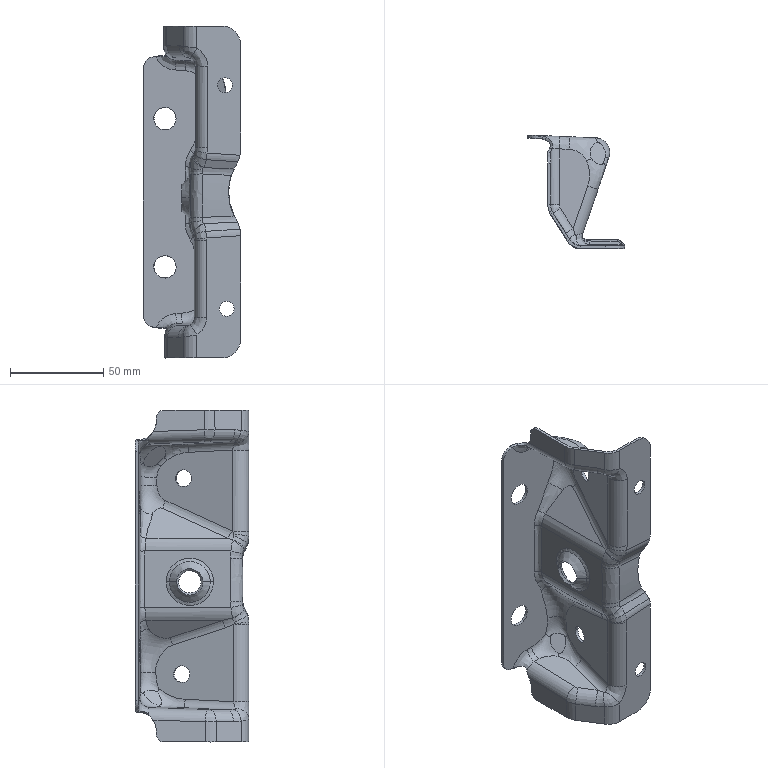Part | STEP file | FNA5401911 | 1 solid | 236 faces | box 52.06 x 60.819 x 178.002 mm | volume 29929 mm3 | spline 140 | cylinder 53 | plane 38 | other 5 | commonest cylinder face diameters 13 x9 10 x6 12 x6 8 x5 9 x4 14 x4